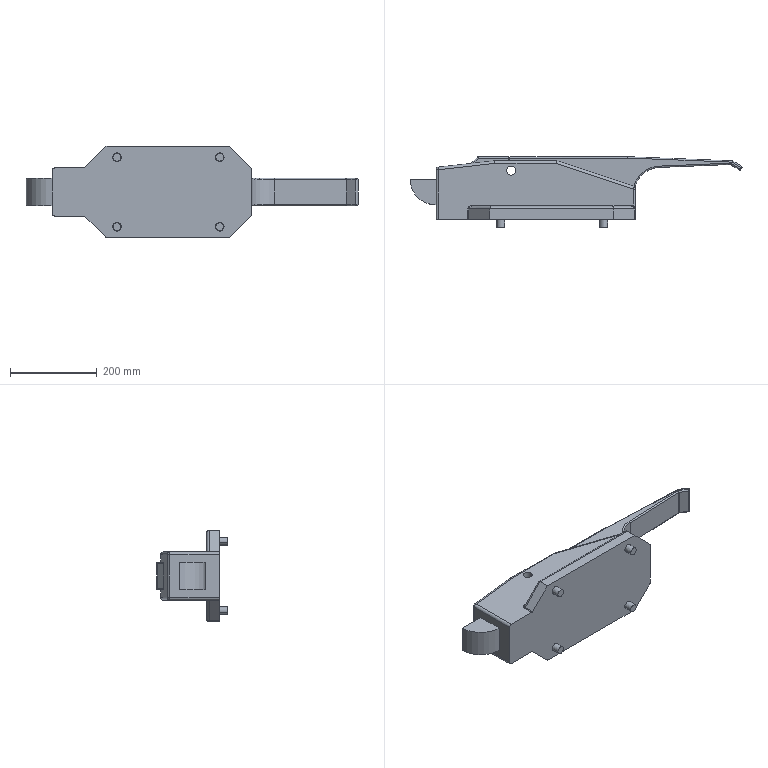Part | SolidWorks | features BaseBody 5, Scale 1 | 5 solids | 236 faces | box 765.696 x 162.57 x 210 mm | volume 8155717 mm3 | cylinder 96 | plane 94 | cone 16 | sphere 14 | spline 10 | torus 6 | commonest cylinder face diameters 6 x35 12 x17 1.8 x16 18 x8 19.8 x8 32.61 x8